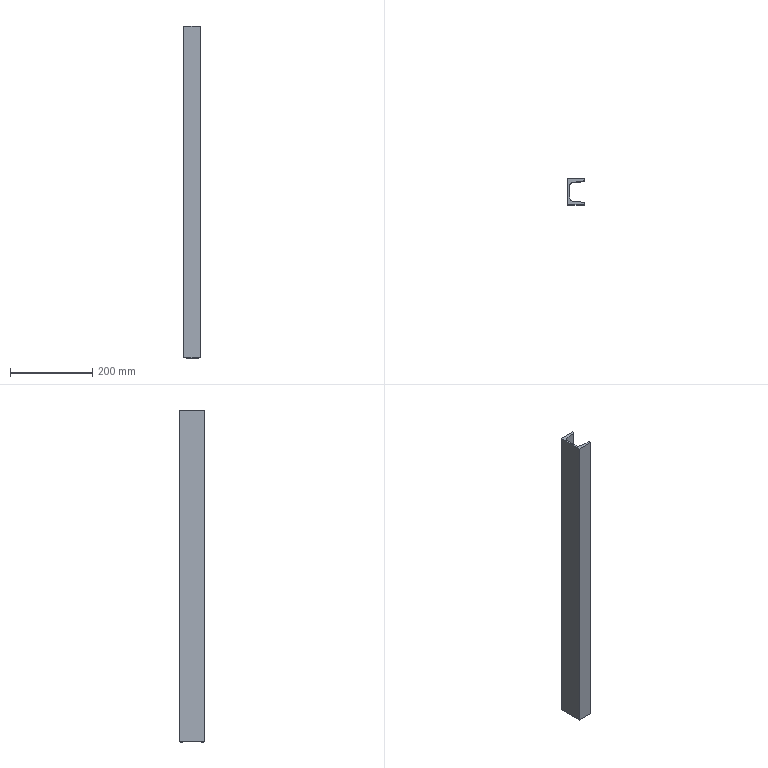Part | STEP file | 750038447 | 1 solid | 32 faces | box 40 x 63 x 809.6 mm | volume 679680 mm3 | plane 18 | cylinder 14 | commonest cylinder face diameters 11 x10 7.6 x2 15 x2
STEP:
#1=CARTESIAN_POINT('',(29.5,56.21,136.));
#2=VERTEX_POINT('',#1);
#3=CARTESIAN_POINT('',(24.,55.66,141.5));
#4=VERTEX_POINT('',#3);
#5=CARTESIAN_POINT('',(29.5,56.21,136.));
#6=CARTESIAN_POINT('',(29.5,56.21,139.222));
#7=CARTESIAN_POINT('',(27.222,55.982,141.5));
#8=CARTESIAN_POINT('',(24.,55.66,141.5));
#9=(BOUNDED_CURVE()B_SPLINE_CURVE(3,(#5,#6,#7,#8),.UNSPECIFIED.,.F.,.T.)B_SPLINE_CURVE_WITH_KNOTS((4,4),(0.,1.571),.UNSPECIFIED.)CURVE()GEOMETRIC_REPRESENTATION_ITEM()RATIONAL_B_SPLINE_CURVE((1.,0.8047,0.8047,1.))REPRESENTATION_ITEM(''));
#10=EDGE_CURVE('',#2,#4,#9,.T.);
#11=ORIENTED_EDGE('',*,*,#10,.T.);
#12=CARTESIAN_POINT('',(24.,63.,141.5));
#13=VERTEX_POINT('',#12);
#14=CARTESIAN_POINT('',(24.,48.,141.5));
#15=DIRECTION('',(0.,1.,0.));
#16=VECTOR('',#15,1000.);
#17=LINE('',#14,#16);
#18=EDGE_CURVE('',#4,#13,#17,.T.);
#19=ORIENTED_EDGE('',*,*,#18,.T.);
#20=CARTESIAN_POINT('',(29.5,63.,136.));
#21=VERTEX_POINT('',#20);
#22=CARTESIAN_POINT('',(24.,63.,136.));
#23=DIRECTION('',(0.,1.,0.));
#24=DIRECTION('',(0.,0.,1.));
#25=AXIS2_PLACEMENT_3D('',#22,#23,#24);
#26=CIRCLE('',#25,5.5);
#27=EDGE_CURVE('',#13,#21,#26,.T.);
#28=ORIENTED_EDGE('',*,*,#27,.T.);
#29=CARTESIAN_POINT('',(29.5,48.,136.));
#30=DIRECTION('',(0.,1.,0.));
#31=VECTOR('',#30,1000.);
#32=LINE('',#29,#31);
#33=EDGE_CURVE('',#2,#21,#32,.T.);
#34=ORIENTED_EDGE('',*,*,#33,.F.);
#35=EDGE_LOOP('',(#11,#19,#28,#34));
#36=FACE_OUTER_BOUND('',#35,.T.);
#37=CARTESIAN_POINT('',(24.,48.,136.));
#38=DIRECTION('',(0.,1.,0.));
#39=DIRECTION('',(0.,0.,1.));
#40=AXIS2_PLACEMENT_3D('',#37,#38,#39);
#41=CYLINDRICAL_SURFACE('',#40,5.5);
#42=ADVANCED_FACE('',(#36),#41,.F.);
#43=CARTESIAN_POINT('',(29.5,56.21,-132.));
#44=VERTEX_POINT('',#43);
#45=CARTESIAN_POINT('',(24.,55.66,-126.5));
#46=VERTEX_POINT('',#45);
#47=CARTESIAN_POINT('',(29.5,56.21,-132.));
#48=CARTESIAN_POINT('',(29.5,56.21,-128.778));
#49=CARTESIAN_POINT('',(27.222,55.982,-126.5));
#50=CARTESIAN_POINT('',(24.,55.66,-126.5));
#51=(BOUNDED_CURVE()B_SPLINE_CURVE(3,(#47,#48,#49,#50),.UNSPECIFIED.,.F.,.F.)B_SPLINE_CURVE_WITH_KNOTS((4,4),(0.,1.571),.UNSPECIFIED.)CURVE()GEOMETRIC_REPRESENTATION_ITEM()RATIONAL_B_SPLINE_CURVE((1.,0.8047,0.8047,1.))REPRESENTATION_ITEM(''));
#52=EDGE_CURVE('',#44,#46,#51,.T.);
#53=ORIENTED_EDGE('',*,*,#52,.T.);
#54=CARTESIAN_POINT('',(24.,63.,-126.5));
#55=VERTEX_POINT('',#54);
#56=CARTESIAN_POINT('',(24.,48.,-126.5));
#57=DIRECTION('',(0.,1.,0.));
#58=VECTOR('',#57,1000.);
#59=LINE('',#56,#58);
#60=EDGE_CURVE('',#46,#55,#59,.T.);
#61=ORIENTED_EDGE('',*,*,#60,.T.);
#62=CARTESIAN_POINT('',(29.5,63.,-132.));
#63=VERTEX_POINT('',#62);
#64=CARTESIAN_POINT('',(24.,63.,-132.));
#65=DIRECTION('',(0.,1.,0.));
#66=DIRECTION('',(0.,0.,1.));
#67=AXIS2_PLACEMENT_3D('',#64,#65,#66);
#68=CIRCLE('',#67,5.5);
#69=EDGE_CURVE('',#55,#63,#68,.T.);
#70=ORIENTED_EDGE('',*,*,#69,.T.);
#71=CARTESIAN_POINT('',(29.5,48.,-132.));
#72=DIRECTION('',(0.,1.,0.));
#73=VECTOR('',#72,1000.);
#74=LINE('',#71,#73);
#75=EDGE_CURVE('',#44,#63,#74,.T.);
#76=ORIENTED_EDGE('',*,*,#75,.F.);
#77=EDGE_LOOP('',(#53,#61,#70,#76));
#78=FACE_OUTER_BOUND('',#77,.T.);
#79=CARTESIAN_POINT('',(24.,48.,-132.));
#80=DIRECTION('',(0.,1.,0.));
#81=DIRECTION('',(0.,0.,1.));
#82=AXIS2_PLACEMENT_3D('',#79,#80,#81);
#83=CYLINDRICAL_SURFACE('',#82,5.5);
#84=ADVANCED_FACE('',(#78),#83,.F.);
#85=CARTESIAN_POINT('',(0.,0.,404.8));
#86=VERTEX_POINT('',#85);
#87=CARTESIAN_POINT('',(0.,0.,-404.8));
#88=VERTEX_POINT('',#87);
#89=CARTESIAN_POINT('',(0.,0.,404.8));
#90=DIRECTION('',(0.,0.,-1.));
#91=VECTOR('',#90,1000.);
#92=LINE('',#89,#91);
#93=EDGE_CURVE('',#86,#88,#92,.T.);
#94=ORIENTED_EDGE('',*,*,#93,.F.);
#95=CARTESIAN_POINT('',(0.,63.,404.8));
#96=VERTEX_POINT('',#95);
#97=CARTESIAN_POINT('',(0.,63.,404.8));
#98=DIRECTION('',(0.,-1.,0.));
#99=VECTOR('',#98,1000.);
#100=LINE('',#97,#99);
#101=EDGE_CURVE('',#96,#86,#100,.T.);
#102=ORIENTED_EDGE('',*,*,#101,.F.);
#103=CARTESIAN_POINT('',(0.,63.,-404.8));
#104=VERTEX_POINT('',#103);
#105=CARTESIAN_POINT('',(0.,63.,404.8));
#106=DIRECTION('',(0.,0.,1.));
#107=VECTOR('',#106,1000.);
#108=LINE('',#105,#107);
#109=EDGE_CURVE('',#104,#96,#108,.T.);
#110=ORIENTED_EDGE('',*,*,#109,.F.);
#111=CARTESIAN_POINT('',(0.,63.,-404.8));
#112=DIRECTION('',(0.,1.,0.));
#113=VECTOR('',#112,1000.);
#114=LINE('',#111,#113);
#115=EDGE_CURVE('',#88,#104,#114,.T.);
#116=ORIENTED_EDGE('',*,*,#115,.F.);
#117=EDGE_LOOP('',(#94,#102,#110,#116));
#118=FACE_OUTER_BOUND('',#117,.T.);
#119=CARTESIAN_POINT('',(0.,63.,404.8));
#120=DIRECTION('',(1.,0.,0.));
#121=DIRECTION('',(0.,0.,-1.));
#122=AXIS2_PLACEMENT_3D('',#119,#120,#121);
#123=PLANE('',#122);
#124=ADVANCED_FACE('',(#118),#123,.F.);
#125=CARTESIAN_POINT('',(40.,63.,-404.8));
#126=VERTEX_POINT('',#125);
#127=CARTESIAN_POINT('',(36.2,63.,-404.8));
#128=DIRECTION('',(-1.,0.,0.));
#129=VECTOR('',#128,1000.);
#130=LINE('',#127,#129);
#131=EDGE_CURVE('',#126,#104,#130,.T.);
#132=ORIENTED_EDGE('',*,*,#131,.F.);
#133=CARTESIAN_POINT('',(40.,60.699,-404.8));
#134=VERTEX_POINT('',#133);
#135=CARTESIAN_POINT('',(40.,2.301,-404.8));
#136=DIRECTION('',(0.,1.,0.));
#137=VECTOR('',#136,1000.);
#138=LINE('',#135,#137);
#139=EDGE_CURVE('',#134,#126,#138,.T.);
#140=ORIENTED_EDGE('',*,*,#139,.F.);
#141=CARTESIAN_POINT('',(36.578,56.918,-404.8));
#142=VERTEX_POINT('',#141);
#143=CARTESIAN_POINT('',(36.2,60.699,-404.8));
#144=DIRECTION('',(0.,0.,1.));
#145=DIRECTION('',(-1.,0.,0.));
#146=AXIS2_PLACEMENT_3D('',#143,#144,#145);
#147=CIRCLE('',#146,3.8);
#148=EDGE_CURVE('',#142,#134,#147,.T.);
#149=ORIENTED_EDGE('',*,*,#148,.F.);
#150=CARTESIAN_POINT('',(11.554,54.415,-404.8));
#151=VERTEX_POINT('',#150);
#152=CARTESIAN_POINT('',(11.554,54.415,-404.8));
#153=DIRECTION('',(0.995,0.0995,0.));
#154=VECTOR('',#153,1000.);
#155=LINE('',#152,#154);
#156=EDGE_CURVE('',#151,#142,#155,.T.);
#157=ORIENTED_EDGE('',*,*,#156,.F.);
#158=CARTESIAN_POINT('',(4.8,46.953,-404.8));
#159=VERTEX_POINT('',#158);
#160=CARTESIAN_POINT('',(12.3,46.953,-404.8));
#161=DIRECTION('',(0.,0.,-1.));
#162=DIRECTION('',(-1.,0.,0.));
#163=AXIS2_PLACEMENT_3D('',#160,#161,#162);
#164=CIRCLE('',#163,7.5);
#165=EDGE_CURVE('',#159,#151,#164,.T.);
#166=ORIENTED_EDGE('',*,*,#165,.F.);
#167=CARTESIAN_POINT('',(4.8,16.047,-404.8));
#168=VERTEX_POINT('',#167);
#169=CARTESIAN_POINT('',(4.8,2.301,-404.8));
#170=DIRECTION('',(0.,1.,0.));
#171=VECTOR('',#170,1000.);
#172=LINE('',#169,#171);
#173=EDGE_CURVE('',#168,#159,#172,.T.);
#174=ORIENTED_EDGE('',*,*,#173,.F.);
#175=CARTESIAN_POINT('',(11.554,8.585,-404.8));
#176=VERTEX_POINT('',#175);
#177=CARTESIAN_POINT('',(12.3,16.047,-404.8));
#178=DIRECTION('',(0.,0.,-1.));
#179=DIRECTION('',(-1.,0.,0.));
#180=AXIS2_PLACEMENT_3D('',#177,#178,#179);
#181=CIRCLE('',#180,7.5);
#182=EDGE_CURVE('',#176,#168,#181,.T.);
#183=ORIENTED_EDGE('',*,*,#182,.F.);
#184=CARTESIAN_POINT('',(36.578,6.082,-404.8));
#185=VERTEX_POINT('',#184);
#186=CARTESIAN_POINT('',(36.578,6.082,-404.8));
#187=DIRECTION('',(-0.995,0.0995,0.));
#188=VECTOR('',#187,1000.);
#189=LINE('',#186,#188);
#190=EDGE_CURVE('',#185,#176,#189,.T.);
#191=ORIENTED_EDGE('',*,*,#190,.F.);
#192=CARTESIAN_POINT('',(40.,2.301,-404.8));
#193=VERTEX_POINT('',#192);
#194=CARTESIAN_POINT('',(36.2,2.301,-404.8));
#195=DIRECTION('',(0.,0.,1.));
#196=DIRECTION('',(-1.,0.,0.));
#197=AXIS2_PLACEMENT_3D('',#194,#195,#196);
#198=CIRCLE('',#197,3.8);
#199=EDGE_CURVE('',#193,#185,#198,.T.);
#200=ORIENTED_EDGE('',*,*,#199,.F.);
#201=CARTESIAN_POINT('',(40.,0.,-404.8));
#202=VERTEX_POINT('',#201);
#203=CARTESIAN_POINT('',(40.,2.301,-404.8));
#204=DIRECTION('',(0.,1.,0.));
#205=VECTOR('',#204,1000.);
#206=LINE('',#203,#205);
#207=EDGE_CURVE('',#202,#193,#206,.T.);
#208=ORIENTED_EDGE('',*,*,#207,.F.);
#209=CARTESIAN_POINT('',(36.2,0.,-404.8));
#210=DIRECTION('',(1.,0.,0.));
#211=VECTOR('',#210,1000.);
#212=LINE('',#209,#211);
#213=EDGE_CURVE('',#88,#202,#212,.T.);
#214=ORIENTED_EDGE('',*,*,#213,.F.);
#215=ORIENTED_EDGE('',*,*,#115,.T.);
#216=EDGE_LOOP('',(#132,#140,#149,#157,#166,#174,#183,#191,#200,#208,#214,#215));
#217=FACE_OUTER_BOUND('',#216,.T.);
#218=CARTESIAN_POINT('',(36.2,2.301,-404.8));
#219=DIRECTION('',(0.,0.,1.));
#220=DIRECTION('',(1.,0.,0.));
#221=AXIS2_PLACEMENT_3D('',#218,#219,#220);
#222=PLANE('',#221);
#223=ADVANCED_FACE('',(#217),#222,.F.);
#224=CARTESIAN_POINT('',(40.,0.,404.8));
#225=VERTEX_POINT('',#224);
#226=CARTESIAN_POINT('',(40.,0.,404.8));
#227=DIRECTION('',(0.,0.,-1.));
#228=VECTOR('',#227,1000.);
#229=LINE('',#226,#228);
#230=EDGE_CURVE('',#225,#202,#229,.T.);
#231=ORIENTED_EDGE('',*,*,#230,.F.);
#232=CARTESIAN_POINT('',(0.,0.,404.8));
#233=DIRECTION('',(1.,0.,0.));
#234=VECTOR('',#233,1000.);
#235=LINE('',#232,#234);
#236=EDGE_CURVE('',#86,#225,#235,.T.);
#237=ORIENTED_EDGE('',*,*,#236,.F.);
#238=ORIENTED_EDGE('',*,*,#93,.T.);
#239=ORIENTED_EDGE('',*,*,#213,.T.);
#240=EDGE_LOOP('',(#231,#237,#238,#239));
#241=FACE_OUTER_BOUND('',#240,.T.);
#242=CARTESIAN_POINT('',(0.,0.,404.8));
#243=DIRECTION('',(0.,1.,0.));
#244=DIRECTION('',(0.,0.,1.));
#245=AXIS2_PLACEMENT_3D('',#242,#243,#244);
#246=PLANE('',#245);
#247=ADVANCED_FACE('',(#241),#246,.F.);
#248=CARTESIAN_POINT('',(40.,60.699,404.8));
#249=VERTEX_POINT('',#248);
#250=CARTESIAN_POINT('',(40.,63.,404.8));
#251=VERTEX_POINT('',#250);
#252=CARTESIAN_POINT('',(40.,2.301,404.8));
#253=DIRECTION('',(0.,1.,0.));
#254=VECTOR('',#253,1000.);
#255=LINE('',#252,#254);
#256=EDGE_CURVE('',#249,#251,#255,.T.);
#257=ORIENTED_EDGE('',*,*,#256,.T.);
#258=CARTESIAN_POINT('',(36.2,63.,404.8));
#259=DIRECTION('',(-1.,0.,0.));
#260=VECTOR('',#259,1000.);
#261=LINE('',#258,#260);
#262=EDGE_CURVE('',#251,#96,#261,.T.);
#263=ORIENTED_EDGE('',*,*,#262,.T.);
#264=ORIENTED_EDGE('',*,*,#101,.T.);
#265=ORIENTED_EDGE('',*,*,#236,.T.);
#266=CARTESIAN_POINT('',(40.,2.301,404.8));
#267=VERTEX_POINT('',#266);
#268=CARTESIAN_POINT('',(40.,2.301,404.8));
#269=DIRECTION('',(0.,1.,0.));
#270=VECTOR('',#269,1000.);
#271=LINE('',#268,#270);
#272=EDGE_CURVE('',#225,#267,#271,.T.);
#273=ORIENTED_EDGE('',*,*,#272,.T.);
#274=CARTESIAN_POINT('',(36.578,6.082,404.8));
#275=VERTEX_POINT('',#274);
#276=CARTESIAN_POINT('',(36.2,2.301,404.8));
#277=DIRECTION('',(0.,0.,1.));
#278=DIRECTION('',(-1.,0.,0.));
#279=AXIS2_PLACEMENT_3D('',#276,#277,#278);
#280=CIRCLE('',#279,3.8);
#281=EDGE_CURVE('',#267,#275,#280,.T.);
#282=ORIENTED_EDGE('',*,*,#281,.T.);
#283=CARTESIAN_POINT('',(11.554,8.585,404.8));
#284=VERTEX_POINT('',#283);
#285=CARTESIAN_POINT('',(36.578,6.082,404.8));
#286=DIRECTION('',(-0.995,0.0995,0.));
#287=VECTOR('',#286,1000.);
#288=LINE('',#285,#287);
#289=EDGE_CURVE('',#275,#284,#288,.T.);
#290=ORIENTED_EDGE('',*,*,#289,.T.);
#291=CARTESIAN_POINT('',(4.8,16.047,404.8));
#292=VERTEX_POINT('',#291);
#293=CARTESIAN_POINT('',(12.3,16.047,404.8));
#294=DIRECTION('',(0.,0.,-1.));
#295=DIRECTION('',(-1.,0.,0.));
#296=AXIS2_PLACEMENT_3D('',#293,#294,#295);
#297=CIRCLE('',#296,7.5);
#298=EDGE_CURVE('',#284,#292,#297,.T.);
#299=ORIENTED_EDGE('',*,*,#298,.T.);
#300=CARTESIAN_POINT('',(4.8,46.953,404.8));
#301=VERTEX_POINT('',#300);
#302=CARTESIAN_POINT('',(4.8,2.301,404.8));
#303=DIRECTION('',(0.,1.,0.));
#304=VECTOR('',#303,1000.);
#305=LINE('',#302,#304);
#306=EDGE_CURVE('',#292,#301,#305,.T.);
#307=ORIENTED_EDGE('',*,*,#306,.T.);
#308=CARTESIAN_POINT('',(11.554,54.415,404.8));
#309=VERTEX_POINT('',#308);
#310=CARTESIAN_POINT('',(12.3,46.953,404.8));
#311=DIRECTION('',(0.,0.,-1.));
#312=DIRECTION('',(-1.,0.,0.));
#313=AXIS2_PLACEMENT_3D('',#310,#311,#312);
#314=CIRCLE('',#313,7.5);
#315=EDGE_CURVE('',#301,#309,#314,.T.);
#316=ORIENTED_EDGE('',*,*,#315,.T.);
#317=CARTESIAN_POINT('',(36.578,56.918,404.8));
#318=VERTEX_POINT('',#317);
#319=CARTESIAN_POINT('',(11.554,54.415,404.8));
#320=DIRECTION('',(0.995,0.0995,0.));
#321=VECTOR('',#320,1000.);
#322=LINE('',#319,#321);
#323=EDGE_CURVE('',#309,#318,#322,.T.);
#324=ORIENTED_EDGE('',*,*,#323,.T.);
#325=CARTESIAN_POINT('',(36.2,60.699,404.8));
#326=DIRECTION('',(0.,0.,1.));
#327=DIRECTION('',(-1.,0.,0.));
#328=AXIS2_PLACEMENT_3D('',#325,#326,#327);
#329=CIRCLE('',#328,3.8);
#330=EDGE_CURVE('',#318,#249,#329,.T.);
#331=ORIENTED_EDGE('',*,*,#330,.T.);
#332=EDGE_LOOP('',(#257,#263,#264,#265,#273,#282,#290,#299,#307,#316,#324,#331));
#333=FACE_OUTER_BOUND('',#332,.T.);
#334=CARTESIAN_POINT('',(36.2,2.301,404.8));
#335=DIRECTION('',(0.,0.,1.));
#336=DIRECTION('',(1.,0.,0.));
#337=AXIS2_PLACEMENT_3D('',#334,#335,#336);
#338=PLANE('',#337);
#339=ADVANCED_FACE('',(#333),#338,.T.);
#340=ORIENTED_EDGE('',*,*,#109,.T.);
#341=ORIENTED_EDGE('',*,*,#262,.F.);
#342=CARTESIAN_POINT('',(40.,63.,404.8));
#343=DIRECTION('',(0.,0.,1.));
#344=VECTOR('',#343,1000.);
#345=LINE('',#342,#344);
#346=EDGE_CURVE('',#126,#251,#345,.T.);
#347=ORIENTED_EDGE('',*,*,#346,.F.);
#348=ORIENTED_EDGE('',*,*,#131,.T.);
#349=EDGE_LOOP('',(#340,#341,#347,#348));
#350=FACE_OUTER_BOUND('',#349,.T.);
#351=CARTESIAN_POINT('',(22.,63.,-171.5));
#352=VERTEX_POINT('',#351);
#353=CARTESIAN_POINT('',(22.,63.,-160.5));
#354=VERTEX_POINT('',#353);
#355=CARTESIAN_POINT('',(22.,63.,-166.));
#356=DIRECTION('',(0.,1.,0.));
#357=DIRECTION('',(0.,0.,1.));
#358=AXIS2_PLACEMENT_3D('',#355,#356,#357);
#359=CIRCLE('',#358,5.5);
#360=EDGE_CURVE('',#352,#354,#359,.T.);
#361=ORIENTED_EDGE('',*,*,#360,.F.);
#362=CARTESIAN_POINT('',(26.,63.,-171.5));
#363=VERTEX_POINT('',#362);
#364=CARTESIAN_POINT('',(40.,63.,-171.5));
#365=DIRECTION('',(-1.,0.,0.));
#366=VECTOR('',#365,1000.);
#367=LINE('',#364,#366);
#368=EDGE_CURVE('',#363,#352,#367,.T.);
#369=ORIENTED_EDGE('',*,*,#368,.F.);
#370=CARTESIAN_POINT('',(26.,63.,-160.5));
#371=VERTEX_POINT('',#370);
#372=CARTESIAN_POINT('',(26.,63.,-166.));
#373=DIRECTION('',(0.,1.,0.));
#374=DIRECTION('',(0.,0.,1.));
#375=AXIS2_PLACEMENT_3D('',#372,#373,#374);
#376=CIRCLE('',#375,5.5);
#377=EDGE_CURVE('',#371,#363,#376,.T.);
#378=ORIENTED_EDGE('',*,*,#377,.F.);
#379=CARTESIAN_POINT('',(40.,63.,-160.5));
#380=DIRECTION('',(1.,0.,0.));
#381=VECTOR('',#380,1000.);
#382=LINE('',#379,#381);
#383=EDGE_CURVE('',#354,#371,#382,.T.);
#384=ORIENTED_EDGE('',*,*,#383,.F.);
#385=EDGE_LOOP('',(#361,#369,#378,#384));
#386=FACE_BOUND('',#385,.T.);
#387=CARTESIAN_POINT('',(18.5,63.,132.));
#388=VERTEX_POINT('',#387);
#389=CARTESIAN_POINT('',(18.5,63.,136.));
#390=VERTEX_POINT('',#389);
#391=CARTESIAN_POINT('',(18.5,63.,404.8));
#392=DIRECTION('',(0.,0.,1.));
#393=VECTOR('',#392,1000.);
#394=LINE('',#391,#393);
#395=EDGE_CURVE('',#388,#390,#394,.T.);
#396=ORIENTED_EDGE('',*,*,#395,.F.);
#397=CARTESIAN_POINT('',(29.5,63.,132.));
#398=VERTEX_POINT('',#397);
#399=CARTESIAN_POINT('',(24.,63.,132.));
#400=DIRECTION('',(0.,1.,0.));
#401=DIRECTION('',(0.,0.,1.));
#402=AXIS2_PLACEMENT_3D('',#399,#400,#401);
#403=CIRCLE('',#402,5.5);
#404=EDGE_CURVE('',#398,#388,#403,.T.);
#405=ORIENTED_EDGE('',*,*,#404,.F.);
#406=CARTESIAN_POINT('',(29.5,63.,404.8));
#407=DIRECTION('',(0.,0.,-1.));
#408=VECTOR('',#407,1000.);
#409=LINE('',#406,#408);
#410=EDGE_CURVE('',#21,#398,#409,.T.);
#411=ORIENTED_EDGE('',*,*,#410,.F.);
#412=ORIENTED_EDGE('',*,*,#27,.F.);
#413=CARTESIAN_POINT('',(24.,63.,136.));
#414=DIRECTION('',(0.,1.,0.));
#415=DIRECTION('',(0.,0.,1.));
#416=AXIS2_PLACEMENT_3D('',#413,#414,#415);
#417=CIRCLE('',#416,5.5);
#418=EDGE_CURVE('',#390,#13,#417,.T.);
#419=ORIENTED_EDGE('',*,*,#418,.F.);
#420=EDGE_LOOP('',(#396,#405,#411,#412,#419));
#421=FACE_BOUND('',#420,.T.);
#422=CARTESIAN_POINT('',(18.5,63.,-136.));
#423=VERTEX_POINT('',#422);
#424=CARTESIAN_POINT('',(18.5,63.,-132.));
#425=VERTEX_POINT('',#424);
#426=CARTESIAN_POINT('',(18.5,63.,404.8));
#427=DIRECTION('',(0.,0.,1.));
#428=VECTOR('',#427,1000.);
#429=LINE('',#426,#428);
#430=EDGE_CURVE('',#423,#425,#429,.T.);
#431=ORIENTED_EDGE('',*,*,#430,.F.);
#432=CARTESIAN_POINT('',(29.5,63.,-136.));
#433=VERTEX_POINT('',#432);
#434=CARTESIAN_POINT('',(24.,63.,-136.));
#435=DIRECTION('',(0.,1.,0.));
#436=DIRECTION('',(0.,0.,1.));
#437=AXIS2_PLACEMENT_3D('',#434,#435,#436);
#438=CIRCLE('',#437,5.5);
#439=EDGE_CURVE('',#433,#423,#438,.T.);
#440=ORIENTED_EDGE('',*,*,#439,.F.);
#441=CARTESIAN_POINT('',(29.5,63.,404.8));
#442=DIRECTION('',(0.,0.,-1.));
#443=VECTOR('',#442,1000.);
#444=LINE('',#441,#443);
#445=EDGE_CURVE('',#63,#433,#444,.T.);
#446=ORIENTED_EDGE('',*,*,#445,.F.);
#447=ORIENTED_EDGE('',*,*,#69,.F.);
#448=CARTESIAN_POINT('',(24.,63.,-132.));
#449=DIRECTION('',(0.,1.,0.));
#450=DIRECTION('',(0.,0.,1.));
#451=AXIS2_PLACEMENT_3D('',#448,#449,#450);
#452=CIRCLE('',#451,5.5);
#453=EDGE_CURVE('',#425,#55,#452,.T.);
#454=ORIENTED_EDGE('',*,*,#453,.F.);
#455=EDGE_LOOP('',(#431,#440,#446,#447,#454));
#456=FACE_BOUND('',#455,.T.);
#457=CARTESIAN_POINT('',(22.,63.,160.5));
#458=VERTEX_POINT('',#457);
#459=CARTESIAN_POINT('',(22.,63.,171.5));
#460=VERTEX_POINT('',#459);
#461=CARTESIAN_POINT('',(22.,63.,166.));
#462=DIRECTION('',(0.,1.,0.));
#463=DIRECTION('',(0.,0.,1.));
#464=AXIS2_PLACEMENT_3D('',#461,#462,#463);
#465=CIRCLE('',#464,5.5);
#466=EDGE_CURVE('',#458,#460,#465,.T.);
#467=ORIENTED_EDGE('',*,*,#466,.F.);
#468=CARTESIAN_POINT('',(26.,63.,160.5));
#469=VERTEX_POINT('',#468);
#470=CARTESIAN_POINT('',(40.,63.,160.5));
#471=DIRECTION('',(-1.,0.,0.));
#472=VECTOR('',#471,1000.);
#473=LINE('',#470,#472);
#474=EDGE_CURVE('',#469,#458,#473,.T.);
#475=ORIENTED_EDGE('',*,*,#474,.F.);
#476=CARTESIAN_POINT('',(26.,63.,171.5));
#477=VERTEX_POINT('',#476);
#478=CARTESIAN_POINT('',(26.,63.,166.));
#479=DIRECTION('',(0.,1.,0.));
#480=DIRECTION('',(0.,0.,1.));
#481=AXIS2_PLACEMENT_3D('',#478,#479,#480);
#482=CIRCLE('',#481,5.5);
#483=EDGE_CURVE('',#477,#469,#482,.T.);
#484=ORIENTED_EDGE('',*,*,#483,.F.);
#485=CARTESIAN_POINT('',(40.,63.,171.5));
#486=DIRECTION('',(1.,0.,0.));
#487=VECTOR('',#486,1000.);
#488=LINE('',#485,#487);
#489=EDGE_CURVE('',#460,#477,#488,.T.);
#490=ORIENTED_EDGE('',*,*,#489,.F.);
#491=EDGE_LOOP('',(#467,#475,#484,#490));
#492=FACE_BOUND('',#491,.T.);
#493=CARTESIAN_POINT('',(40.,63.,404.8));
#494=DIRECTION('',(0.,-1.,0.));
#495=DIRECTION('',(0.,0.,-1.));
#496=AXIS2_PLACEMENT_3D('',#493,#494,#495);
#497=PLANE('',#496);
#498=ADVANCED_FACE('',(#350,#386,#421,#456,#492),#497,.F.);
#499=ORIENTED_EDGE('',*,*,#346,.T.);
#500=ORIENTED_EDGE('',*,*,#256,.F.);
#501=CARTESIAN_POINT('',(40.,60.699,404.8));
#502=DIRECTION('',(0.,0.,1.));
#503=VECTOR('',#502,1000.);
#504=LINE('',#501,#503);
#505=EDGE_CURVE('',#134,#249,#504,.T.);
#506=ORIENTED_EDGE('',*,*,#505,.F.);
#507=ORIENTED_EDGE('',*,*,#139,.T.);
#508=EDGE_LOOP('',(#499,#500,#506,#507));
#509=FACE_OUTER_BOUND('',#508,.T.);
#510=CARTESIAN_POINT('',(40.,60.699,404.8));
#511=DIRECTION('',(-1.,0.,0.));
#512=DIRECTION('',(0.,-1.,0.));
#513=AXIS2_PLACEMENT_3D('',#510,#511,#512);
#514=PLANE('',#513);
#515=ADVANCED_FACE('',(#509),#514,.F.);
#516=ORIENTED_EDGE('',*,*,#330,.F.);
#517=CARTESIAN_POINT('',(36.578,56.918,404.8));
#518=DIRECTION('',(0.,0.,-1.));
#519=VECTOR('',#518,1000.);
#520=LINE('',#517,#519);
#521=EDGE_CURVE('',#318,#142,#520,.T.);
#522=ORIENTED_EDGE('',*,*,#521,.T.);
#523=ORIENTED_EDGE('',*,*,#148,.T.);
#524=ORIENTED_EDGE('',*,*,#505,.T.);
#525=EDGE_LOOP('',(#516,#522,#523,#524));
#526=FACE_OUTER_BOUND('',#525,.T.);
#527=CARTESIAN_POINT('',(36.2,60.699,404.8));
#528=DIRECTION('',(0.,0.,-1.));
#529=DIRECTION('',(-1.,0.,0.));
#530=AXIS2_PLACEMENT_3D('',#527,#528,#529);
#531=CYLINDRICAL_SURFACE('',#530,3.8);
#532=ADVANCED_FACE('',(#526),#531,.T.);
#533=ORIENTED_EDGE('',*,*,#521,.F.);
#534=ORIENTED_EDGE('',*,*,#323,.F.);
#535=CARTESIAN_POINT('',(11.554,54.415,404.8));
#536=DIRECTION('',(0.,0.,1.));
#537=VECTOR('',#536,1000.);
#538=LINE('',#535,#537);
#539=EDGE_CURVE('',#151,#309,#538,.T.);
#540=ORIENTED_EDGE('',*,*,#539,.F.);
#541=ORIENTED_EDGE('',*,*,#156,.T.);
#542=EDGE_LOOP('',(#533,#534,#540,#541));
#543=FACE_OUTER_BOUND('',#542,.T.);
#544=CARTESIAN_POINT('',(22.,55.46,-160.5));
#545=VERTEX_POINT('',#544);
#546=CARTESIAN_POINT('',(22.,55.46,-171.5));
#547=VERTEX_POINT('',#546);
#548=CARTESIAN_POINT('',(22.,55.46,-160.5));
#549=CARTESIAN_POINT('',(11.,54.36,-160.5));
#550=CARTESIAN_POINT('',(11.,54.36,-171.5));
#551=CARTESIAN_POINT('',(22.,55.46,-171.5));
#552=(BOUNDED_CURVE()B_SPLINE_CURVE(3,(#548,#549,#550,#551),.UNSPECIFIED.,.F.,.F.)B_SPLINE_CURVE_WITH_KNOTS((4,4),(1.571,4.712),.UNSPECIFIED.)CURVE()GEOMETRIC_REPRESENTATION_ITEM()RATIONAL_B_SPLINE_CURVE((1.,0.3333,0.3333,1.))REPRESENTATION_ITEM(''));
#553=EDGE_CURVE('',#545,#547,#552,.T.);
#554=ORIENTED_EDGE('',*,*,#553,.F.);
#555=CARTESIAN_POINT('',(26.,55.86,-160.5));
#556=VERTEX_POINT('',#555);
#557=CARTESIAN_POINT('',(11.554,54.415,-160.5));
#558=DIRECTION('',(-0.995,-0.0995,0.));
#559=VECTOR('',#558,1000.);
#560=LINE('',#557,#559);
#561=EDGE_CURVE('',#556,#545,#560,.T.);
#562=ORIENTED_EDGE('',*,*,#561,.F.);
#563=CARTESIAN_POINT('',(26.,55.86,-171.5));
#564=VERTEX_POINT('',#563);
#565=CARTESIAN_POINT('',(26.,55.86,-171.5));
#566=CARTESIAN_POINT('',(37.,56.96,-171.5));
#567=CARTESIAN_POINT('',(37.,56.96,-160.5));
#568=CARTESIAN_POINT('',(26.,55.86,-160.5));
#569=(BOUNDED_CURVE()B_SPLINE_CURVE(3,(#565,#566,#567,#568),.UNSPECIFIED.,.F.,.F.)B_SPLINE_CURVE_WITH_KNOTS((4,4),(4.712,7.854),.UNSPECIFIED.)CURVE()GEOMETRIC_REPRESENTATION_ITEM()RATIONAL_B_SPLINE_CURVE((1.,0.3333,0.3333,1.))REPRESENTATION_ITEM(''));
#570=EDGE_CURVE('',#564,#556,#569,.T.);
#571=ORIENTED_EDGE('',*,*,#570,.F.);
#572=CARTESIAN_POINT('',(11.554,54.415,-171.5));
#573=DIRECTION('',(0.995,0.0995,0.));
#574=VECTOR('',#573,1000.);
#575=LINE('',#572,#574);
#576=EDGE_CURVE('',#547,#564,#575,.T.);
#577=ORIENTED_EDGE('',*,*,#576,.F.);
#578=EDGE_LOOP('',(#554,#562,#571,#577));
#579=FACE_BOUND('',#578,.T.);
#580=CARTESIAN_POINT('',(18.5,55.11,136.));
#581=VERTEX_POINT('',#580);
#582=CARTESIAN_POINT('',(18.5,55.11,132.));
#583=VERTEX_POINT('',#582);
#584=CARTESIAN_POINT('',(18.5,55.11,404.8));
#585=DIRECTION('',(0.,0.,-1.));
#586=VECTOR('',#585,1000.);
#587=LINE('',#584,#586);
#588=EDGE_CURVE('',#581,#583,#587,.T.);
#589=ORIENTED_EDGE('',*,*,#588,.F.);
#590=CARTESIAN_POINT('',(24.,55.66,141.5));
#591=CARTESIAN_POINT('',(20.778,55.338,141.5));
#592=CARTESIAN_POINT('',(18.5,55.11,139.222));
#593=CARTESIAN_POINT('',(18.5,55.11,136.));
#594=(BOUNDED_CURVE()B_SPLINE_CURVE(3,(#590,#591,#592,#593),.UNSPECIFIED.,.F.,.F.)B_SPLINE_CURVE_WITH_KNOTS((4,4),(1.571,3.142),.UNSPECIFIED.)CURVE()GEOMETRIC_REPRESENTATION_ITEM()RATIONAL_B_SPLINE_CURVE((1.,0.8047,0.8047,1.))REPRESENTATION_ITEM(''));
#595=EDGE_CURVE('',#4,#581,#594,.T.);
#596=ORIENTED_EDGE('',*,*,#595,.F.);
#597=ORIENTED_EDGE('',*,*,#10,.F.);
#598=CARTESIAN_POINT('',(29.5,56.21,132.));
#599=VERTEX_POINT('',#598);
#600=CARTESIAN_POINT('',(29.5,56.21,404.8));
#601=DIRECTION('',(0.,0.,1.));
#602=VECTOR('',#601,1000.);
#603=LINE('',#600,#602);
#604=EDGE_CURVE('',#599,#2,#603,.T.);
#605=ORIENTED_EDGE('',*,*,#604,.F.);
#606=CARTESIAN_POINT('',(18.5,55.11,132.));
#607=CARTESIAN_POINT('',(18.5,55.11,121.));
#608=CARTESIAN_POINT('',(29.5,56.21,121.));
#609=CARTESIAN_POINT('',(29.5,56.21,132.));
#610=(BOUNDED_CURVE()B_SPLINE_CURVE(3,(#606,#607,#608,#609),.UNSPECIFIED.,.F.,.F.)B_SPLINE_CURVE_WITH_KNOTS((4,4),(3.142,6.283),.UNSPECIFIED.)CURVE()GEOMETRIC_REPRESENTATION_ITEM()RATIONAL_B_SPLINE_CURVE((1.,0.3333,0.3333,1.))REPRESENTATION_ITEM(''));
#611=EDGE_CURVE('',#583,#599,#610,.T.);
#612=ORIENTED_EDGE('',*,*,#611,.F.);
#613=EDGE_LOOP('',(#589,#596,#597,#605,#612));
#614=FACE_BOUND('',#613,.T.);
#615=CARTESIAN_POINT('',(18.5,55.11,-132.));
#616=VERTEX_POINT('',#615);
#617=CARTESIAN_POINT('',(18.5,55.11,-136.));
#618=VERTEX_POINT('',#617);
#619=CARTESIAN_POINT('',(18.5,55.11,404.8));
#620=DIRECTION('',(0.,0.,-1.));
#621=VECTOR('',#620,1000.);
#622=LINE('',#619,#621);
#623=EDGE_CURVE('',#616,#618,#622,.T.);
#624=ORIENTED_EDGE('',*,*,#623,.F.);
#625=CARTESIAN_POINT('',(24.,55.66,-126.5));
#626=CARTESIAN_POINT('',(20.778,55.338,-126.5));
#627=CARTESIAN_POINT('',(18.5,55.11,-128.778));
#628=CARTESIAN_POINT('',(18.5,55.11,-132.));
#629=(BOUNDED_CURVE()B_SPLINE_CURVE(3,(#625,#626,#627,#628),.UNSPECIFIED.,.F.,.F.)B_SPLINE_CURVE_WITH_KNOTS((4,4),(1.571,3.142),.UNSPECIFIED.)CURVE()GEOMETRIC_REPRESENTATION_ITEM()RATIONAL_B_SPLINE_CURVE((1.,0.8047,0.8047,1.))REPRESENTATION_ITEM(''));
#630=EDGE_CURVE('',#46,#616,#629,.T.);
#631=ORIENTED_EDGE('',*,*,#630,.F.);
#632=ORIENTED_EDGE('',*,*,#52,.F.);
#633=CARTESIAN_POINT('',(29.5,56.21,-136.));
#634=VERTEX_POINT('',#633);
#635=CARTESIAN_POINT('',(29.5,56.21,404.8));
#636=DIRECTION('',(0.,0.,1.));
#637=VECTOR('',#636,1000.);
#638=LINE('',#635,#637);
#639=EDGE_CURVE('',#634,#44,#638,.T.);
#640=ORIENTED_EDGE('',*,*,#639,.F.);
#641=CARTESIAN_POINT('',(18.5,55.11,-136.));
#642=CARTESIAN_POINT('',(18.5,55.11,-147.));
#643=CARTESIAN_POINT('',(29.5,56.21,-147.));
#644=CARTESIAN_POINT('',(29.5,56.21,-136.));
#645=(BOUNDED_CURVE()B_SPLINE_CURVE(3,(#641,#642,#643,#644),.UNSPECIFIED.,.F.,.T.)B_SPLINE_CURVE_WITH_KNOTS((4,4),(3.142,6.283),.UNSPECIFIED.)CURVE()GEOMETRIC_REPRESENTATION_ITEM()RATIONAL_B_SPLINE_CURVE((1.,0.3333,0.3333,1.))REPRESENTATION_ITEM(''));
#646=EDGE_CURVE('',#618,#634,#645,.T.);
#647=ORIENTED_EDGE('',*,*,#646,.F.);
#648=EDGE_LOOP('',(#624,#631,#632,#640,#647));
#649=FACE_BOUND('',#648,.T.);
#650=CARTESIAN_POINT('',(22.,55.46,171.5));
#651=VERTEX_POINT('',#650);
#652=CARTESIAN_POINT('',(22.,55.46,160.5));
#653=VERTEX_POINT('',#652);
#654=CARTESIAN_POINT('',(22.,55.46,171.5));
#655=CARTESIAN_POINT('',(11.,54.36,171.5));
#656=CARTESIAN_POINT('',(11.,54.36,160.5));
#657=CARTESIAN_POINT('',(22.,55.46,160.5));
#658=(BOUNDED_CURVE()B_SPLINE_CURVE(3,(#654,#655,#656,#657),.UNSPECIFIED.,.F.,.T.)B_SPLINE_CURVE_WITH_KNOTS((4,4),(1.571,4.712),.UNSPECIFIED.)CURVE()GEOMETRIC_REPRESENTATION_ITEM()RATIONAL_B_SPLINE_CURVE((1.,0.3333,0.3333,1.))REPRESENTATION_ITEM(''));
#659=EDGE_CURVE('',#651,#653,#658,.T.);
#660=ORIENTED_EDGE('',*,*,#659,.F.);
#661=CARTESIAN_POINT('',(26.,55.86,171.5));
#662=VERTEX_POINT('',#661);
#663=CARTESIAN_POINT('',(11.554,54.415,171.5));
#664=DIRECTION('',(-0.995,-0.0995,0.));
#665=VECTOR('',#664,1000.);
#666=LINE('',#663,#665);
#667=EDGE_CURVE('',#662,#651,#666,.T.);
#668=ORIENTED_EDGE('',*,*,#667,.F.);
#669=CARTESIAN_POINT('',(26.,55.86,160.5));
#670=VERTEX_POINT('',#669);
#671=CARTESIAN_POINT('',(26.,55.86,160.5));
#672=CARTESIAN_POINT('',(37.,56.96,160.5));
#673=CARTESIAN_POINT('',(37.,56.96,171.5));
#674=CARTESIAN_POINT('',(26.,55.86,171.5));
#675=(BOUNDED_CURVE()B_SPLINE_CURVE(3,(#671,#672,#673,#674),.UNSPECIFIED.,.F.,.F.)B_SPLINE_CURVE_WITH_KNOTS((4,4),(4.712,7.854),.UNSPECIFIED.)CURVE()GEOMETRIC_REPRESENTATION_ITEM()RATIONAL_B_SPLINE_CURVE((1.,0.3333,0.3333,1.))REPRESENTATION_ITEM(''));
#676=EDGE_CURVE('',#670,#662,#675,.T.);
#677=ORIENTED_EDGE('',*,*,#676,.F.);
#678=CARTESIAN_POINT('',(11.554,54.415,160.5));
#679=DIRECTION('',(0.995,0.0995,0.));
#680=VECTOR('',#679,1000.);
#681=LINE('',#678,#680);
#682=EDGE_CURVE('',#653,#670,#681,.T.);
#683=ORIENTED_EDGE('',*,*,#682,.F.);
#684=EDGE_LOOP('',(#660,#668,#677,#683));
#685=FACE_BOUND('',#684,.T.);
#686=CARTESIAN_POINT('',(11.554,54.415,404.8));
#687=DIRECTION('',(-0.0995,0.995,0.));
#688=DIRECTION('',(-0.995,-0.0995,0.));
#689=AXIS2_PLACEMENT_3D('',#686,#687,#688);
#690=PLANE('',#689);
#691=ADVANCED_FACE('',(#543,#579,#614,#649,#685),#690,.F.);
#692=ORIENTED_EDGE('',*,*,#539,.T.);
#693=ORIENTED_EDGE('',*,*,#315,.F.);
#694=CARTESIAN_POINT('',(4.8,46.953,404.8));
#695=DIRECTION('',(0.,0.,1.));
#696=VECTOR('',#695,1000.);
#697=LINE('',#694,#696);
#698=EDGE_CURVE('',#159,#301,#697,.T.);
#699=ORIENTED_EDGE('',*,*,#698,.F.);
#700=ORIENTED_EDGE('',*,*,#165,.T.);
#701=EDGE_LOOP('',(#692,#693,#699,#700));
#702=FACE_OUTER_BOUND('',#701,.T.);
#703=CARTESIAN_POINT('',(12.3,46.953,404.8));
#704=DIRECTION('',(0.,0.,-1.));
#705=DIRECTION('',(-1.,0.,0.));
#706=AXIS2_PLACEMENT_3D('',#703,#704,#705);
#707=CYLINDRICAL_SURFACE('',#706,7.5);
#708=ADVANCED_FACE('',(#702),#707,.F.);
#709=ORIENTED_EDGE('',*,*,#698,.T.);
#710=ORIENTED_EDGE('',*,*,#306,.F.);
#711=CARTESIAN_POINT('',(4.8,16.047,404.8));
#712=DIRECTION('',(0.,0.,1.));
#713=VECTOR('',#712,1000.);
#714=LINE('',#711,#713);
#715=EDGE_CURVE('',#168,#292,#714,.T.);
#716=ORIENTED_EDGE('',*,*,#715,.F.);
#717=ORIENTED_EDGE('',*,*,#173,.T.);
#718=EDGE_LOOP('',(#709,#710,#716,#717));
#719=FACE_OUTER_BOUND('',#718,.T.);
#720=CARTESIAN_POINT('',(4.8,16.047,404.8));
#721=DIRECTION('',(-1.,0.,0.));
#722=DIRECTION('',(0.,-1.,0.));
#723=AXIS2_PLACEMENT_3D('',#720,#721,#722);
#724=PLANE('',#723);
#725=ADVANCED_FACE('',(#719),#724,.F.);
#726=ORIENTED_EDGE('',*,*,#715,.T.);
#727=ORIENTED_EDGE('',*,*,#298,.F.);
#728=CARTESIAN_POINT('',(11.554,8.585,404.8));
#729=DIRECTION('',(0.,0.,1.));
#730=VECTOR('',#729,1000.);
#731=LINE('',#728,#730);
#732=EDGE_CURVE('',#176,#284,#731,.T.);
#733=ORIENTED_EDGE('',*,*,#732,.F.);
#734=ORIENTED_EDGE('',*,*,#182,.T.);
#735=EDGE_LOOP('',(#726,#727,#733,#734));
#736=FACE_OUTER_BOUND('',#735,.T.);
#737=CARTESIAN_POINT('',(12.3,16.047,404.8));
#738=DIRECTION('',(0.,0.,-1.));
#739=DIRECTION('',(-1.,0.,0.));
#740=AXIS2_PLACEMENT_3D('',#737,#738,#739);
#741=CYLINDRICAL_SURFACE('',#740,7.5);
#742=ADVANCED_FACE('',(#736),#741,.F.);
#743=ORIENTED_EDGE('',*,*,#732,.T.);
#744=ORIENTED_EDGE('',*,*,#289,.F.);
#745=CARTESIAN_POINT('',(36.578,6.082,404.8));
#746=DIRECTION('',(0.,0.,1.));
#747=VECTOR('',#746,1000.);
#748=LINE('',#745,#747);
#749=EDGE_CURVE('',#185,#275,#748,.T.);
#750=ORIENTED_EDGE('',*,*,#749,.F.);
#751=ORIENTED_EDGE('',*,*,#190,.T.);
#752=EDGE_LOOP('',(#743,#744,#750,#751));
#753=FACE_OUTER_BOUND('',#752,.T.);
#754=CARTESIAN_POINT('',(36.578,6.082,404.8));
#755=DIRECTION('',(-0.0995,-0.995,0.));
#756=DIRECTION('',(0.995,-0.0995,0.));
#757=AXIS2_PLACEMENT_3D('',#754,#755,#756);
#758=PLANE('',#757);
#759=ADVANCED_FACE('',(#753),#758,.F.);
#760=ORIENTED_EDGE('',*,*,#281,.F.);
#761=CARTESIAN_POINT('',(40.,2.301,404.8));
#762=DIRECTION('',(0.,0.,-1.));
#763=VECTOR('',#762,1000.);
#764=LINE('',#761,#763);
#765=EDGE_CURVE('',#267,#193,#764,.T.);
#766=ORIENTED_EDGE('',*,*,#765,.T.);
#767=ORIENTED_EDGE('',*,*,#199,.T.);
#768=ORIENTED_EDGE('',*,*,#749,.T.);
#769=EDGE_LOOP('',(#760,#766,#767,#768));
#770=FACE_OUTER_BOUND('',#769,.T.);
#771=CARTESIAN_POINT('',(36.2,2.301,404.8));
#772=DIRECTION('',(0.,0.,-1.));
#773=DIRECTION('',(-1.,0.,0.));
#774=AXIS2_PLACEMENT_3D('',#771,#772,#773);
#775=CYLINDRICAL_SURFACE('',#774,3.8);
#776=ADVANCED_FACE('',(#770),#775,.T.);
#777=ORIENTED_EDGE('',*,*,#765,.F.);
#778=ORIENTED_EDGE('',*,*,#272,.F.);
#779=ORIENTED_EDGE('',*,*,#230,.T.);
#780=ORIENTED_EDGE('',*,*,#207,.T.);
#781=EDGE_LOOP('',(#777,#778,#779,#780));
#782=FACE_OUTER_BOUND('',#781,.T.);
#783=CARTESIAN_POINT('',(40.,0.,404.8));
#784=DIRECTION('',(-1.,0.,0.));
#785=DIRECTION('',(0.,0.,1.));
#786=AXIS2_PLACEMENT_3D('',#783,#784,#785);
#787=PLANE('',#786);
#788=ADVANCED_FACE('',(#782),#787,.F.);
#789=ORIENTED_EDGE('',*,*,#383,.T.);
#790=CARTESIAN_POINT('',(26.,48.,-160.5));
#791=DIRECTION('',(0.,1.,0.));
#792=VECTOR('',#791,1000.);
#793=LINE('',#790,#792);
#794=EDGE_CURVE('',#556,#371,#793,.T.);
#795=ORIENTED_EDGE('',*,*,#794,.F.);
#796=ORIENTED_EDGE('',*,*,#561,.T.);
#797=CARTESIAN_POINT('',(22.,48.,-160.5));
#798=DIRECTION('',(0.,-1.,0.));
#799=VECTOR('',#798,1000.);
#800=LINE('',#797,#799);
#801=EDGE_CURVE('',#354,#545,#800,.T.);
#802=ORIENTED_EDGE('',*,*,#801,.F.);
#803=EDGE_LOOP('',(#789,#795,#796,#802));
#804=FACE_OUTER_BOUND('',#803,.T.);
#805=CARTESIAN_POINT('',(22.,48.,-160.5));
#806=DIRECTION('',(0.,0.,1.));
#807=DIRECTION('',(1.,0.,0.));
#808=AXIS2_PLACEMENT_3D('',#805,#806,#807);
#809=PLANE('',#808);
#810=ADVANCED_FACE('',(#804),#809,.F.);
#811=ORIENTED_EDGE('',*,*,#360,.T.);
#812=ORIENTED_EDGE('',*,*,#801,.T.);
#813=ORIENTED_EDGE('',*,*,#553,.T.);
#814=CARTESIAN_POINT('',(22.,48.,-171.5));
#815=DIRECTION('',(0.,-1.,0.));
#816=VECTOR('',#815,1000.);
#817=LINE('',#814,#816);
#818=EDGE_CURVE('',#352,#547,#817,.T.);
#819=ORIENTED_EDGE('',*,*,#818,.F.);
#820=EDGE_LOOP('',(#811,#812,#813,#819));
#821=FACE_OUTER_BOUND('',#820,.T.);
#822=CARTESIAN_POINT('',(22.,48.,-166.));
#823=DIRECTION('',(0.,1.,0.));
#824=DIRECTION('',(0.,0.,1.));
#825=AXIS2_PLACEMENT_3D('',#822,#823,#824);
#826=CYLINDRICAL_SURFACE('',#825,5.5);
#827=ADVANCED_FACE('',(#821),#826,.F.);
#828=ORIENTED_EDGE('',*,*,#368,.T.);
#829=ORIENTED_EDGE('',*,*,#818,.T.);
#830=ORIENTED_EDGE('',*,*,#576,.T.);
#831=CARTESIAN_POINT('',(26.,48.,-171.5));
#832=DIRECTION('',(0.,-1.,0.));
#833=VECTOR('',#832,1000.);
#834=LINE('',#831,#833);
#835=EDGE_CURVE('',#363,#564,#834,.T.);
#836=ORIENTED_EDGE('',*,*,#835,.F.);
#837=EDGE_LOOP('',(#828,#829,#830,#836));
#838=FACE_OUTER_BOUND('',#837,.T.);
#839=CARTESIAN_POINT('',(26.,48.,-171.5));
#840=DIRECTION('',(0.,0.,-1.));
#841=DIRECTION('',(-1.,0.,0.));
#842=AXIS2_PLACEMENT_3D('',#839,#840,#841);
#843=PLANE('',#842);
#844=ADVANCED_FACE('',(#838),#843,.F.);
#845=ORIENTED_EDGE('',*,*,#377,.T.);
#846=ORIENTED_EDGE('',*,*,#835,.T.);
#847=ORIENTED_EDGE('',*,*,#570,.T.);
#848=ORIENTED_EDGE('',*,*,#794,.T.);
#849=EDGE_LOOP('',(#845,#846,#847,#848));
#850=FACE_OUTER_BOUND('',#849,.T.);
#851=CARTESIAN_POINT('',(26.,48.,-166.));
#852=DIRECTION('',(0.,1.,0.));
#853=DIRECTION('',(0.,0.,1.));
#854=AXIS2_PLACEMENT_3D('',#851,#852,#853);
#855=CYLINDRICAL_SURFACE('',#854,5.5);
#856=ADVANCED_FACE('',(#850),#855,.F.);
#857=ORIENTED_EDGE('',*,*,#18,.F.);
#858=ORIENTED_EDGE('',*,*,#595,.T.);
#859=CARTESIAN_POINT('',(18.5,48.,136.));
#860=DIRECTION('',(0.,-1.,0.));
#861=VECTOR('',#860,1000.);
#862=LINE('',#859,#861);
#863=EDGE_CURVE('',#390,#581,#862,.T.);
#864=ORIENTED_EDGE('',*,*,#863,.F.);
#865=ORIENTED_EDGE('',*,*,#418,.T.);
#866=EDGE_LOOP('',(#857,#858,#864,#865));
#867=FACE_OUTER_BOUND('',#866,.T.);
#868=CARTESIAN_POINT('',(24.,48.,136.));
#869=DIRECTION('',(0.,1.,0.));
#870=DIRECTION('',(0.,0.,1.));
#871=AXIS2_PLACEMENT_3D('',#868,#869,#870);
#872=CYLINDRICAL_SURFACE('',#871,5.5);
#873=ADVANCED_FACE('',(#867),#872,.F.);
#874=ORIENTED_EDGE('',*,*,#395,.T.);
#875=ORIENTED_EDGE('',*,*,#863,.T.);
#876=ORIENTED_EDGE('',*,*,#588,.T.);
#877=CARTESIAN_POINT('',(18.5,48.,132.));
#878=DIRECTION('',(0.,-1.,0.));
#879=VECTOR('',#878,1000.);
#880=LINE('',#877,#879);
#881=EDGE_CURVE('',#388,#583,#880,.T.);
#882=ORIENTED_EDGE('',*,*,#881,.F.);
#883=EDGE_LOOP('',(#874,#875,#876,#882));
#884=FACE_OUTER_BOUND('',#883,.T.);
#885=CARTESIAN_POINT('',(18.5,48.,132.));
#886=DIRECTION('',(-1.,0.,0.));
#887=DIRECTION('',(0.,0.,1.));
#888=AXIS2_PLACEMENT_3D('',#885,#886,#887);
#889=PLANE('',#888);
#890=ADVANCED_FACE('',(#884),#889,.F.);
#891=ORIENTED_EDGE('',*,*,#404,.T.);
#892=ORIENTED_EDGE('',*,*,#881,.T.);
#893=ORIENTED_EDGE('',*,*,#611,.T.);
#894=CARTESIAN_POINT('',(29.5,48.,132.));
#895=DIRECTION('',(0.,-1.,0.));
#896=VECTOR('',#895,1000.);
#897=LINE('',#894,#896);
#898=EDGE_CURVE('',#398,#599,#897,.T.);
#899=ORIENTED_EDGE('',*,*,#898,.F.);
#900=EDGE_LOOP('',(#891,#892,#893,#899));
#901=FACE_OUTER_BOUND('',#900,.T.);
#902=CARTESIAN_POINT('',(24.,48.,132.));
#903=DIRECTION('',(0.,1.,0.));
#904=DIRECTION('',(0.,0.,1.));
#905=AXIS2_PLACEMENT_3D('',#902,#903,#904);
#906=CYLINDRICAL_SURFACE('',#905,5.5);
#907=ADVANCED_FACE('',(#901),#906,.F.);
#908=ORIENTED_EDGE('',*,*,#410,.T.);
#909=ORIENTED_EDGE('',*,*,#898,.T.);
#910=ORIENTED_EDGE('',*,*,#604,.T.);
#911=ORIENTED_EDGE('',*,*,#33,.T.);
#912=EDGE_LOOP('',(#908,#909,#910,#911));
#913=FACE_OUTER_BOUND('',#912,.T.);
#914=CARTESIAN_POINT('',(29.5,48.,136.));
#915=DIRECTION('',(1.,0.,0.));
#916=DIRECTION('',(0.,0.,-1.));
#917=AXIS2_PLACEMENT_3D('',#914,#915,#916);
#918=PLANE('',#917);
#919=ADVANCED_FACE('',(#913),#918,.F.);
#920=ORIENTED_EDGE('',*,*,#60,.F.);
#921=ORIENTED_EDGE('',*,*,#630,.T.);
#922=CARTESIAN_POINT('',(18.5,48.,-132.));
#923=DIRECTION('',(0.,-1.,0.));
#924=VECTOR('',#923,1000.);
#925=LINE('',#922,#924);
#926=EDGE_CURVE('',#425,#616,#925,.T.);
#927=ORIENTED_EDGE('',*,*,#926,.F.);
#928=ORIENTED_EDGE('',*,*,#453,.T.);
#929=EDGE_LOOP('',(#920,#921,#927,#928));
#930=FACE_OUTER_BOUND('',#929,.T.);
#931=CARTESIAN_POINT('',(24.,48.,-132.));
#932=DIRECTION('',(0.,1.,0.));
#933=DIRECTION('',(0.,0.,1.));
#934=AXIS2_PLACEMENT_3D('',#931,#932,#933);
#935=CYLINDRICAL_SURFACE('',#934,5.5);
#936=ADVANCED_FACE('',(#930),#935,.F.);
#937=ORIENTED_EDGE('',*,*,#430,.T.);
#938=ORIENTED_EDGE('',*,*,#926,.T.);
#939=ORIENTED_EDGE('',*,*,#623,.T.);
#940=CARTESIAN_POINT('',(18.5,48.,-136.));
#941=DIRECTION('',(0.,-1.,0.));
#942=VECTOR('',#941,1000.);
#943=LINE('',#940,#942);
#944=EDGE_CURVE('',#423,#618,#943,.T.);
#945=ORIENTED_EDGE('',*,*,#944,.F.);
#946=EDGE_LOOP('',(#937,#938,#939,#945));
#947=FACE_OUTER_BOUND('',#946,.T.);
#948=CARTESIAN_POINT('',(18.5,48.,-136.));
#949=DIRECTION('',(-1.,0.,0.));
#950=DIRECTION('',(0.,0.,1.));
#951=AXIS2_PLACEMENT_3D('',#948,#949,#950);
#952=PLANE('',#951);
#953=ADVANCED_FACE('',(#947),#952,.F.);
#954=ORIENTED_EDGE('',*,*,#439,.T.);
#955=ORIENTED_EDGE('',*,*,#944,.T.);
#956=ORIENTED_EDGE('',*,*,#646,.T.);
#957=CARTESIAN_POINT('',(29.5,48.,-136.));
#958=DIRECTION('',(0.,-1.,0.));
#959=VECTOR('',#958,1000.);
#960=LINE('',#957,#959);
#961=EDGE_CURVE('',#433,#634,#960,.T.);
#962=ORIENTED_EDGE('',*,*,#961,.F.);
#963=EDGE_LOOP('',(#954,#955,#956,#962));
#964=FACE_OUTER_BOUND('',#963,.T.);
#965=CARTESIAN_POINT('',(24.,48.,-136.));
#966=DIRECTION('',(0.,1.,0.));
#967=DIRECTION('',(0.,0.,1.));
#968=AXIS2_PLACEMENT_3D('',#965,#966,#967);
#969=CYLINDRICAL_SURFACE('',#968,5.5);
#970=ADVANCED_FACE('',(#964),#969,.F.);
#971=ORIENTED_EDGE('',*,*,#445,.T.);
#972=ORIENTED_EDGE('',*,*,#961,.T.);
#973=ORIENTED_EDGE('',*,*,#639,.T.);
#974=ORIENTED_EDGE('',*,*,#75,.T.);
#975=EDGE_LOOP('',(#971,#972,#973,#974));
#976=FACE_OUTER_BOUND('',#975,.T.);
#977=CARTESIAN_POINT('',(29.5,48.,-132.));
#978=DIRECTION('',(1.,0.,0.));
#979=DIRECTION('',(0.,0.,-1.));
#980=AXIS2_PLACEMENT_3D('',#977,#978,#979);
#981=PLANE('',#980);
#982=ADVANCED_FACE('',(#976),#981,.F.);
#983=ORIENTED_EDGE('',*,*,#489,.T.);
#984=CARTESIAN_POINT('',(26.,48.,171.5));
#985=DIRECTION('',(0.,1.,0.));
#986=VECTOR('',#985,1000.);
#987=LINE('',#984,#986);
#988=EDGE_CURVE('',#662,#477,#987,.T.);
#989=ORIENTED_EDGE('',*,*,#988,.F.);
#990=ORIENTED_EDGE('',*,*,#667,.T.);
#991=CARTESIAN_POINT('',(22.,48.,171.5));
#992=DIRECTION('',(0.,-1.,0.));
#993=VECTOR('',#992,1000.);
#994=LINE('',#991,#993);
#995=EDGE_CURVE('',#460,#651,#994,.T.);
#996=ORIENTED_EDGE('',*,*,#995,.F.);
#997=EDGE_LOOP('',(#983,#989,#990,#996));
#998=FACE_OUTER_BOUND('',#997,.T.);
#999=CARTESIAN_POINT('',(22.,48.,171.5));
#1000=DIRECTION('',(0.,0.,1.));
#1001=DIRECTION('',(1.,0.,0.));
#1002=AXIS2_PLACEMENT_3D('',#999,#1000,#1001);
#1003=PLANE('',#1002);
#1004=ADVANCED_FACE('',(#998),#1003,.F.);
#1005=ORIENTED_EDGE('',*,*,#466,.T.);
#1006=ORIENTED_EDGE('',*,*,#995,.T.);
#1007=ORIENTED_EDGE('',*,*,#659,.T.);
#1008=CARTESIAN_POINT('',(22.,48.,160.5));
#1009=DIRECTION('',(0.,-1.,0.));
#1010=VECTOR('',#1009,1000.);
#1011=LINE('',#1008,#1010);
#1012=EDGE_CURVE('',#458,#653,#1011,.T.);
#1013=ORIENTED_EDGE('',*,*,#1012,.F.);
#1014=EDGE_LOOP('',(#1005,#1006,#1007,#1013));
#1015=FACE_OUTER_BOUND('',#1014,.T.);
#1016=CARTESIAN_POINT('',(22.,48.,166.));
#1017=DIRECTION('',(0.,1.,0.));
#1018=DIRECTION('',(0.,0.,1.));
#1019=AXIS2_PLACEMENT_3D('',#1016,#1017,#1018);
#1020=CYLINDRICAL_SURFACE('',#1019,5.5);
#1021=ADVANCED_FACE('',(#1015),#1020,.F.);
#1022=ORIENTED_EDGE('',*,*,#474,.T.);
#1023=ORIENTED_EDGE('',*,*,#1012,.T.);
#1024=ORIENTED_EDGE('',*,*,#682,.T.);
#1025=CARTESIAN_POINT('',(26.,48.,160.5));
#1026=DIRECTION('',(0.,-1.,0.));
#1027=VECTOR('',#1026,1000.);
#1028=LINE('',#1025,#1027);
#1029=EDGE_CURVE('',#469,#670,#1028,.T.);
#1030=ORIENTED_EDGE('',*,*,#1029,.F.);
#1031=EDGE_LOOP('',(#1022,#1023,#1024,#1030));
#1032=FACE_OUTER_BOUND('',#1031,.T.);
#1033=CARTESIAN_POINT('',(26.,48.,160.5));
#1034=DIRECTION('',(0.,0.,-1.));
#1035=DIRECTION('',(-1.,0.,0.));
#1036=AXIS2_PLACEMENT_3D('',#1033,#1034,#1035);
#1037=PLANE('',#1036);
#1038=ADVANCED_FACE('',(#1032),#1037,.F.);
#1039=ORIENTED_EDGE('',*,*,#483,.T.);
#1040=ORIENTED_EDGE('',*,*,#1029,.T.);
#1041=ORIENTED_EDGE('',*,*,#676,.T.);
#1042=ORIENTED_EDGE('',*,*,#988,.T.);
#1043=EDGE_LOOP('',(#1039,#1040,#1041,#1042));
#1044=FACE_OUTER_BOUND('',#1043,.T.);
#1045=CARTESIAN_POINT('',(26.,48.,166.));
#1046=DIRECTION('',(0.,1.,0.));
#1047=DIRECTION('',(0.,0.,1.));
#1048=AXIS2_PLACEMENT_3D('',#1045,#1046,#1047);
#1049=CYLINDRICAL_SURFACE('',#1048,5.5);
#1050=ADVANCED_FACE('',(#1044),#1049,.F.);
#1051=CLOSED_SHELL('',(#42,#84,#124,#223,#247,#339,#498,#515,#532,#691,#708,#725,#742,#759,#776,#788,#810,#827,#844,#856,#873,#890,#907,#919,#936,#953,#970,#982,#1004,#1021,#1038,#1050));
#1052=MANIFOLD_SOLID_BREP('',#1051);
#1053=CARTESIAN_POINT('',(0.,0.,0.));
#1054=DIRECTION('',(0.,0.,1.));
#1055=DIRECTION('',(1.,0.,0.));
#1056=AXIS2_PLACEMENT_3D('',#1053,#1054,#1055);
#1057=(LENGTH_UNIT()NAMED_UNIT(*)SI_UNIT(.MILLI.,.METRE.));
#1058=UNCERTAINTY_MEASURE_WITH_UNIT(LENGTH_MEASURE(0.00001),#1057,'','');
#1059=(NAMED_UNIT(*)PLANE_ANGLE_UNIT()SI_UNIT($,.RADIAN.));
#1060=(NAMED_UNIT(*)SI_UNIT($,.STERADIAN.)SOLID_ANGLE_UNIT());
#1061=(GEOMETRIC_REPRESENTATION_CONTEXT(3)GLOBAL_UNCERTAINTY_ASSIGNED_CONTEXT((#1058))GLOBAL_UNIT_ASSIGNED_CONTEXT((#1057,#1059,#1060))REPRESENTATION_CONTEXT('',''));
#1062=ADVANCED_BREP_SHAPE_REPRESENTATION('',(#1052,#1056),#1061);